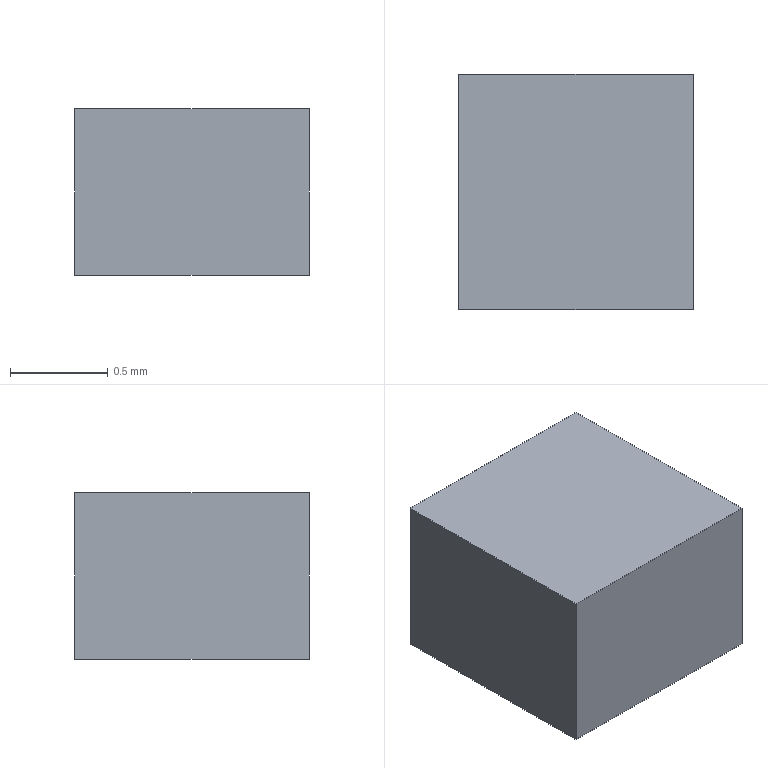Part | Creo | 1 solid | 6 faces | box 1.2 x 1.2 x 0.8485 mm | volume 1.222 mm3 | plane 6
STEP:
#1=CARTESIAN_POINT('',(0.,0.,0.));
#2=DIRECTION('',(0.,0.,1.));
#3=DIRECTION('',(1.,0.,0.));
#4=AXIS2_PLACEMENT_3D('',#1,#2,#3);
#5=CARTESIAN_POINT('',(-0.6,-0.6,0.));
#6=VERTEX_POINT('',#5);
#7=CARTESIAN_POINT('',(0.6,-0.6,0.));
#8=VERTEX_POINT('',#7);
#9=CARTESIAN_POINT('',(-0.6,-0.6,0.));
#10=DIRECTION('',(1.,0.,0.));
#11=VECTOR('',#10,1.2);
#12=LINE('',#9,#11);
#13=EDGE_CURVE('',#6,#8,#12,.T.);
#14=ORIENTED_EDGE('',*,*,#13,.T.);
#15=CARTESIAN_POINT('',(0.6,0.6,0.));
#16=VERTEX_POINT('',#15);
#17=CARTESIAN_POINT('',(0.6,-0.6,0.));
#18=DIRECTION('',(0.,1.,0.));
#19=VECTOR('',#18,1.2);
#20=LINE('',#17,#19);
#21=EDGE_CURVE('',#8,#16,#20,.T.);
#22=ORIENTED_EDGE('',*,*,#21,.T.);
#23=CARTESIAN_POINT('',(-0.6,0.6,0.));
#24=VERTEX_POINT('',#23);
#25=CARTESIAN_POINT('',(0.6,0.6,0.));
#26=DIRECTION('',(-1.,0.,0.));
#27=VECTOR('',#26,1.2);
#28=LINE('',#25,#27);
#29=EDGE_CURVE('',#16,#24,#28,.T.);
#30=ORIENTED_EDGE('',*,*,#29,.T.);
#31=CARTESIAN_POINT('',(-0.6,0.6,0.));
#32=DIRECTION('',(0.,-1.,0.));
#33=VECTOR('',#32,1.2);
#34=LINE('',#31,#33);
#35=EDGE_CURVE('',#24,#6,#34,.T.);
#36=ORIENTED_EDGE('',*,*,#35,.T.);
#37=EDGE_LOOP('',(#14,#22,#30,#36));
#38=FACE_OUTER_BOUND('',#37,.F.);
#39=CARTESIAN_POINT('',(0.,0.,0.));
#40=DIRECTION('',(0.,0.,1.));
#41=DIRECTION('',(1.,0.,0.));
#42=AXIS2_PLACEMENT_3D('',#39,#40,#41);
#43=PLANE('',#42);
#44=ADVANCED_FACE('',(#38),#43,.F.);
#45=ORIENTED_EDGE('',*,*,#13,.F.);
#46=CARTESIAN_POINT('',(-0.6,-0.6,0.8485));
#47=VERTEX_POINT('',#46);
#48=CARTESIAN_POINT('',(-0.6,-0.6,0.));
#49=DIRECTION('',(0.,0.,1.));
#50=VECTOR('',#49,0.8485);
#51=LINE('',#48,#50);
#52=EDGE_CURVE('',#6,#47,#51,.T.);
#53=ORIENTED_EDGE('',*,*,#52,.T.);
#54=CARTESIAN_POINT('',(0.6,-0.6,0.8485));
#55=VERTEX_POINT('',#54);
#56=CARTESIAN_POINT('',(-0.6,-0.6,0.8485));
#57=DIRECTION('',(1.,0.,0.));
#58=VECTOR('',#57,1.2);
#59=LINE('',#56,#58);
#60=EDGE_CURVE('',#47,#55,#59,.T.);
#61=ORIENTED_EDGE('',*,*,#60,.T.);
#62=CARTESIAN_POINT('',(0.6,-0.6,0.));
#63=DIRECTION('',(0.,0.,1.));
#64=VECTOR('',#63,0.8485);
#65=LINE('',#62,#64);
#66=EDGE_CURVE('',#8,#55,#65,.T.);
#67=ORIENTED_EDGE('',*,*,#66,.F.);
#68=EDGE_LOOP('',(#45,#53,#61,#67));
#69=FACE_OUTER_BOUND('',#68,.F.);
#70=CARTESIAN_POINT('',(-0.6,-0.6,0.));
#71=DIRECTION('',(0.,-1.,0.));
#72=DIRECTION('',(1.,0.,0.));
#73=AXIS2_PLACEMENT_3D('',#70,#71,#72);
#74=PLANE('',#73);
#75=ADVANCED_FACE('',(#69),#74,.T.);
#76=ORIENTED_EDGE('',*,*,#35,.F.);
#77=CARTESIAN_POINT('',(-0.6,0.6,0.8485));
#78=VERTEX_POINT('',#77);
#79=CARTESIAN_POINT('',(-0.6,0.6,0.));
#80=DIRECTION('',(0.,0.,1.));
#81=VECTOR('',#80,0.8485);
#82=LINE('',#79,#81);
#83=EDGE_CURVE('',#24,#78,#82,.T.);
#84=ORIENTED_EDGE('',*,*,#83,.T.);
#85=CARTESIAN_POINT('',(-0.6,0.6,0.8485));
#86=DIRECTION('',(0.,-1.,0.));
#87=VECTOR('',#86,1.2);
#88=LINE('',#85,#87);
#89=EDGE_CURVE('',#78,#47,#88,.T.);
#90=ORIENTED_EDGE('',*,*,#89,.T.);
#91=ORIENTED_EDGE('',*,*,#52,.F.);
#92=EDGE_LOOP('',(#76,#84,#90,#91));
#93=FACE_OUTER_BOUND('',#92,.F.);
#94=CARTESIAN_POINT('',(-0.6,0.6,0.));
#95=DIRECTION('',(-1.,0.,0.));
#96=DIRECTION('',(0.,-1.,0.));
#97=AXIS2_PLACEMENT_3D('',#94,#95,#96);
#98=PLANE('',#97);
#99=ADVANCED_FACE('',(#93),#98,.T.);
#100=ORIENTED_EDGE('',*,*,#29,.F.);
#101=CARTESIAN_POINT('',(0.6,0.6,0.8485));
#102=VERTEX_POINT('',#101);
#103=CARTESIAN_POINT('',(0.6,0.6,0.));
#104=DIRECTION('',(0.,0.,1.));
#105=VECTOR('',#104,0.8485);
#106=LINE('',#103,#105);
#107=EDGE_CURVE('',#16,#102,#106,.T.);
#108=ORIENTED_EDGE('',*,*,#107,.T.);
#109=CARTESIAN_POINT('',(0.6,0.6,0.8485));
#110=DIRECTION('',(-1.,0.,0.));
#111=VECTOR('',#110,1.2);
#112=LINE('',#109,#111);
#113=EDGE_CURVE('',#102,#78,#112,.T.);
#114=ORIENTED_EDGE('',*,*,#113,.T.);
#115=ORIENTED_EDGE('',*,*,#83,.F.);
#116=EDGE_LOOP('',(#100,#108,#114,#115));
#117=FACE_OUTER_BOUND('',#116,.F.);
#118=CARTESIAN_POINT('',(0.6,0.6,0.));
#119=DIRECTION('',(0.,1.,0.));
#120=DIRECTION('',(-1.,0.,0.));
#121=AXIS2_PLACEMENT_3D('',#118,#119,#120);
#122=PLANE('',#121);
#123=ADVANCED_FACE('',(#117),#122,.T.);
#124=ORIENTED_EDGE('',*,*,#21,.F.);
#125=ORIENTED_EDGE('',*,*,#66,.T.);
#126=CARTESIAN_POINT('',(0.6,-0.6,0.8485));
#127=DIRECTION('',(0.,1.,0.));
#128=VECTOR('',#127,1.2);
#129=LINE('',#126,#128);
#130=EDGE_CURVE('',#55,#102,#129,.T.);
#131=ORIENTED_EDGE('',*,*,#130,.T.);
#132=ORIENTED_EDGE('',*,*,#107,.F.);
#133=EDGE_LOOP('',(#124,#125,#131,#132));
#134=FACE_OUTER_BOUND('',#133,.F.);
#135=CARTESIAN_POINT('',(0.6,-0.6,0.));
#136=DIRECTION('',(1.,0.,0.));
#137=DIRECTION('',(0.,1.,0.));
#138=AXIS2_PLACEMENT_3D('',#135,#136,#137);
#139=PLANE('',#138);
#140=ADVANCED_FACE('',(#134),#139,.T.);
#141=ORIENTED_EDGE('',*,*,#60,.F.);
#142=ORIENTED_EDGE('',*,*,#89,.F.);
#143=ORIENTED_EDGE('',*,*,#113,.F.);
#144=ORIENTED_EDGE('',*,*,#130,.F.);
#145=EDGE_LOOP('',(#141,#142,#143,#144));
#146=FACE_OUTER_BOUND('',#145,.F.);
#147=CARTESIAN_POINT('',(0.,0.,0.8485));
#148=DIRECTION('',(0.,0.,1.));
#149=DIRECTION('',(1.,0.,0.));
#150=AXIS2_PLACEMENT_3D('',#147,#148,#149);
#151=PLANE('',#150);
#152=ADVANCED_FACE('',(#146),#151,.T.);
#153=CLOSED_SHELL('',(#44,#75,#99,#123,#140,#152));
#154=MANIFOLD_SOLID_BREP('',#153);
#155=(LENGTH_UNIT()NAMED_UNIT(*)SI_UNIT(.MILLI.,.METRE.));
#156=UNCERTAINTY_MEASURE_WITH_UNIT(LENGTH_MEASURE(0.0001897),#155,'','');
#157=(NAMED_UNIT(*)PLANE_ANGLE_UNIT()SI_UNIT($,.RADIAN.));
#158=PLANE_ANGLE_MEASURE_WITH_UNIT(PLANE_ANGLE_MEASURE(0.01745),#157);
#159=(CONVERSION_BASED_UNIT('DEGREE',#158)NAMED_UNIT(*)PLANE_ANGLE_UNIT());
#160=(NAMED_UNIT(*)SI_UNIT($,.STERADIAN.)SOLID_ANGLE_UNIT());
#161=(GEOMETRIC_REPRESENTATION_CONTEXT(3)GLOBAL_UNCERTAINTY_ASSIGNED_CONTEXT((#156))GLOBAL_UNIT_ASSIGNED_CONTEXT((#155,#159,#160))REPRESENTATION_CONTEXT('',''));
#162=ADVANCED_BREP_SHAPE_REPRESENTATION('',(#4,#154),#161);